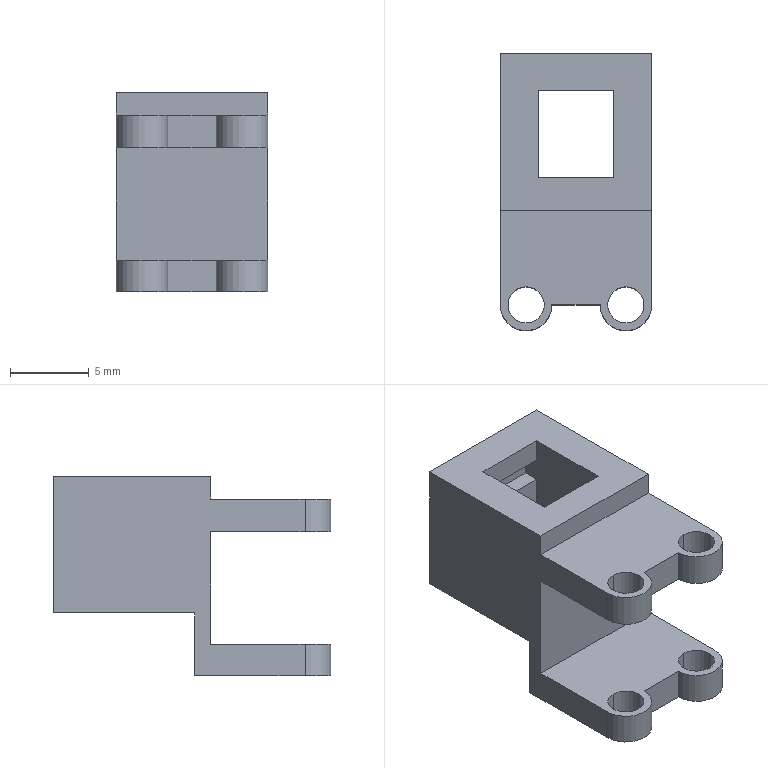Part | SolidWorks | features ICE 8, Extrusion 1 | 1 solid | 38 faces | box 9.63 x 17.64 x 12.7 mm | volume 865.254 mm3 | plane 26 | cylinder 12 | commonest cylinder face diameters 2.3 x8 3.28 x4
STEP:
#1=CARTESIAN_POINT('',(0.,1.15,7.242));
#2=VERTEX_POINT('',#1);
#3=CARTESIAN_POINT('',(0.,-1.15,7.242));
#4=VERTEX_POINT('',#3);
#5=CARTESIAN_POINT('',(0.,0.,7.242));
#6=DIRECTION('',(0.,0.,1.));
#7=DIRECTION('',(1.,0.,0.));
#8=AXIS2_PLACEMENT_3D('',#5,#6,#7);
#9=CIRCLE('',#8,1.15);
#10=EDGE_CURVE('',#2,#4,#9,.T.);
#11=ORIENTED_EDGE('',*,*,#10,.T.);
#12=CARTESIAN_POINT('',(0.,-1.15,5.171));
#13=VERTEX_POINT('',#12);
#14=CARTESIAN_POINT('',(0.,-1.15,8.7));
#15=DIRECTION('',(0.,0.,-1.));
#16=VECTOR('',#15,1000.);
#17=LINE('',#14,#16);
#18=EDGE_CURVE('',#4,#13,#17,.T.);
#19=ORIENTED_EDGE('',*,*,#18,.T.);
#20=CARTESIAN_POINT('',(0.,1.15,5.171));
#21=VERTEX_POINT('',#20);
#22=CARTESIAN_POINT('',(0.,0.,5.171));
#23=DIRECTION('',(0.,0.,-1.));
#24=DIRECTION('',(-1.,0.,0.));
#25=AXIS2_PLACEMENT_3D('',#22,#23,#24);
#26=CIRCLE('',#25,1.15);
#27=EDGE_CURVE('',#13,#21,#26,.T.);
#28=ORIENTED_EDGE('',*,*,#27,.T.);
#29=CARTESIAN_POINT('',(0.,1.15,8.7));
#30=DIRECTION('',(0.,0.,-1.));
#31=VECTOR('',#30,1000.);
#32=LINE('',#29,#31);
#33=EDGE_CURVE('',#2,#21,#32,.T.);
#34=ORIENTED_EDGE('',*,*,#33,.F.);
#35=EDGE_LOOP('',(#11,#19,#28,#34));
#36=FACE_OUTER_BOUND('',#35,.T.);
#37=CARTESIAN_POINT('',(0.,0.,8.7));
#38=DIRECTION('',(0.,0.,-1.));
#39=DIRECTION('',(0.,1.,0.));
#40=AXIS2_PLACEMENT_3D('',#37,#38,#39);
#41=CYLINDRICAL_SURFACE('',#40,1.15);
#42=ADVANCED_FACE('',(#36),#41,.F.);
#43=CARTESIAN_POINT('',(-6.35,1.15,7.242));
#44=VERTEX_POINT('',#43);
#45=CARTESIAN_POINT('',(-6.35,-1.15,7.242));
#46=VERTEX_POINT('',#45);
#47=CARTESIAN_POINT('',(-6.35,0.,7.242));
#48=DIRECTION('',(0.,0.,1.));
#49=DIRECTION('',(1.,0.,0.));
#50=AXIS2_PLACEMENT_3D('',#47,#48,#49);
#51=CIRCLE('',#50,1.15);
#52=EDGE_CURVE('',#44,#46,#51,.T.);
#53=ORIENTED_EDGE('',*,*,#52,.T.);
#54=CARTESIAN_POINT('',(-6.35,-1.15,5.171));
#55=VERTEX_POINT('',#54);
#56=CARTESIAN_POINT('',(-6.35,-1.15,8.7));
#57=DIRECTION('',(0.,0.,-1.));
#58=VECTOR('',#57,1000.);
#59=LINE('',#56,#58);
#60=EDGE_CURVE('',#46,#55,#59,.T.);
#61=ORIENTED_EDGE('',*,*,#60,.T.);
#62=CARTESIAN_POINT('',(-6.35,1.15,5.171));
#63=VERTEX_POINT('',#62);
#64=CARTESIAN_POINT('',(-6.35,0.,5.171));
#65=DIRECTION('',(0.,0.,-1.));
#66=DIRECTION('',(-1.,0.,0.));
#67=AXIS2_PLACEMENT_3D('',#64,#65,#66);
#68=CIRCLE('',#67,1.15);
#69=EDGE_CURVE('',#55,#63,#68,.T.);
#70=ORIENTED_EDGE('',*,*,#69,.T.);
#71=CARTESIAN_POINT('',(-6.35,1.15,8.7));
#72=DIRECTION('',(0.,0.,-1.));
#73=VECTOR('',#72,1000.);
#74=LINE('',#71,#73);
#75=EDGE_CURVE('',#44,#63,#74,.T.);
#76=ORIENTED_EDGE('',*,*,#75,.F.);
#77=EDGE_LOOP('',(#53,#61,#70,#76));
#78=FACE_OUTER_BOUND('',#77,.T.);
#79=CARTESIAN_POINT('',(-6.35,0.,8.7));
#80=DIRECTION('',(0.,0.,-1.));
#81=DIRECTION('',(0.,1.,0.));
#82=AXIS2_PLACEMENT_3D('',#79,#80,#81);
#83=CYLINDRICAL_SURFACE('',#82,1.15);
#84=ADVANCED_FACE('',(#78),#83,.F.);
#85=CARTESIAN_POINT('',(0.,1.15,-2.));
#86=VERTEX_POINT('',#85);
#87=CARTESIAN_POINT('',(0.,-1.15,-2.));
#88=VERTEX_POINT('',#87);
#89=CARTESIAN_POINT('',(0.,0.,-2.));
#90=DIRECTION('',(0.,0.,1.));
#91=DIRECTION('',(0.,-1.,0.));
#92=AXIS2_PLACEMENT_3D('',#89,#90,#91);
#93=CIRCLE('',#92,1.15);
#94=EDGE_CURVE('',#86,#88,#93,.T.);
#95=ORIENTED_EDGE('',*,*,#94,.T.);
#96=CARTESIAN_POINT('',(0.,-1.15,-4.));
#97=VERTEX_POINT('',#96);
#98=CARTESIAN_POINT('',(0.,-1.15,8.7));
#99=DIRECTION('',(0.,0.,-1.));
#100=VECTOR('',#99,1000.);
#101=LINE('',#98,#100);
#102=EDGE_CURVE('',#88,#97,#101,.T.);
#103=ORIENTED_EDGE('',*,*,#102,.T.);
#104=CARTESIAN_POINT('',(0.,1.15,-4.));
#105=VERTEX_POINT('',#104);
#106=CARTESIAN_POINT('',(0.,0.,-4.));
#107=DIRECTION('',(0.,0.,-1.));
#108=DIRECTION('',(0.,1.,0.));
#109=AXIS2_PLACEMENT_3D('',#106,#107,#108);
#110=CIRCLE('',#109,1.15);
#111=EDGE_CURVE('',#97,#105,#110,.T.);
#112=ORIENTED_EDGE('',*,*,#111,.T.);
#113=CARTESIAN_POINT('',(0.,1.15,8.7));
#114=DIRECTION('',(0.,0.,-1.));
#115=VECTOR('',#114,1000.);
#116=LINE('',#113,#115);
#117=EDGE_CURVE('',#86,#105,#116,.T.);
#118=ORIENTED_EDGE('',*,*,#117,.F.);
#119=EDGE_LOOP('',(#95,#103,#112,#118));
#120=FACE_OUTER_BOUND('',#119,.T.);
#121=CARTESIAN_POINT('',(0.,0.,8.7));
#122=DIRECTION('',(0.,0.,-1.));
#123=DIRECTION('',(0.,1.,0.));
#124=AXIS2_PLACEMENT_3D('',#121,#122,#123);
#125=CYLINDRICAL_SURFACE('',#124,1.15);
#126=ADVANCED_FACE('',(#120),#125,.F.);
#127=CARTESIAN_POINT('',(-6.35,1.15,-2.));
#128=VERTEX_POINT('',#127);
#129=CARTESIAN_POINT('',(-6.35,-1.15,-2.));
#130=VERTEX_POINT('',#129);
#131=CARTESIAN_POINT('',(-6.35,0.,-2.));
#132=DIRECTION('',(0.,0.,1.));
#133=DIRECTION('',(0.,-1.,0.));
#134=AXIS2_PLACEMENT_3D('',#131,#132,#133);
#135=CIRCLE('',#134,1.15);
#136=EDGE_CURVE('',#128,#130,#135,.T.);
#137=ORIENTED_EDGE('',*,*,#136,.T.);
#138=CARTESIAN_POINT('',(-6.35,-1.15,-4.));
#139=VERTEX_POINT('',#138);
#140=CARTESIAN_POINT('',(-6.35,-1.15,8.7));
#141=DIRECTION('',(0.,0.,-1.));
#142=VECTOR('',#141,1000.);
#143=LINE('',#140,#142);
#144=EDGE_CURVE('',#130,#139,#143,.T.);
#145=ORIENTED_EDGE('',*,*,#144,.T.);
#146=CARTESIAN_POINT('',(-6.35,1.15,-4.));
#147=VERTEX_POINT('',#146);
#148=CARTESIAN_POINT('',(-6.35,0.,-4.));
#149=DIRECTION('',(0.,0.,-1.));
#150=DIRECTION('',(0.,1.,0.));
#151=AXIS2_PLACEMENT_3D('',#148,#149,#150);
#152=CIRCLE('',#151,1.15);
#153=EDGE_CURVE('',#139,#147,#152,.T.);
#154=ORIENTED_EDGE('',*,*,#153,.T.);
#155=CARTESIAN_POINT('',(-6.35,1.15,8.7));
#156=DIRECTION('',(0.,0.,-1.));
#157=VECTOR('',#156,1000.);
#158=LINE('',#155,#157);
#159=EDGE_CURVE('',#128,#147,#158,.T.);
#160=ORIENTED_EDGE('',*,*,#159,.F.);
#161=EDGE_LOOP('',(#137,#145,#154,#160));
#162=FACE_OUTER_BOUND('',#161,.T.);
#163=CARTESIAN_POINT('',(-6.35,0.,8.7));
#164=DIRECTION('',(0.,0.,-1.));
#165=DIRECTION('',(0.,1.,0.));
#166=AXIS2_PLACEMENT_3D('',#163,#164,#165);
#167=CYLINDRICAL_SURFACE('',#166,1.15);
#168=ADVANCED_FACE('',(#162),#167,.F.);
#169=CARTESIAN_POINT('',(0.,0.,5.171));
#170=DIRECTION('',(0.,0.,-1.));
#171=DIRECTION('',(-1.,0.,0.));
#172=AXIS2_PLACEMENT_3D('',#169,#170,#171);
#173=CIRCLE('',#172,1.15);
#174=EDGE_CURVE('',#21,#13,#173,.T.);
#175=ORIENTED_EDGE('',*,*,#174,.F.);
#176=ORIENTED_EDGE('',*,*,#27,.F.);
#177=EDGE_LOOP('',(#175,#176));
#178=FACE_BOUND('',#177,.T.);
#179=CARTESIAN_POINT('',(-6.35,0.,5.171));
#180=DIRECTION('',(0.,0.,-1.));
#181=DIRECTION('',(-1.,0.,0.));
#182=AXIS2_PLACEMENT_3D('',#179,#180,#181);
#183=CIRCLE('',#182,1.15);
#184=EDGE_CURVE('',#63,#55,#183,.T.);
#185=ORIENTED_EDGE('',*,*,#184,.F.);
#186=ORIENTED_EDGE('',*,*,#69,.F.);
#187=EDGE_LOOP('',(#185,#186));
#188=FACE_BOUND('',#187,.T.);
#189=CARTESIAN_POINT('',(1.64,6.,5.171));
#190=VERTEX_POINT('',#189);
#191=CARTESIAN_POINT('',(1.64,0.,5.171));
#192=VERTEX_POINT('',#191);
#193=CARTESIAN_POINT('',(1.64,-1.64,5.171));
#194=DIRECTION('',(0.,-1.,0.));
#195=VECTOR('',#194,1000.);
#196=LINE('',#193,#195);
#197=EDGE_CURVE('',#190,#192,#196,.T.);
#198=ORIENTED_EDGE('',*,*,#197,.T.);
#199=CARTESIAN_POINT('',(-1.64,0.,5.171));
#200=VERTEX_POINT('',#199);
#201=CARTESIAN_POINT('',(0.,0.,5.171));
#202=DIRECTION('',(0.,0.,-1.));
#203=DIRECTION('',(-1.,0.,0.));
#204=AXIS2_PLACEMENT_3D('',#201,#202,#203);
#205=CIRCLE('',#204,1.64);
#206=EDGE_CURVE('',#192,#200,#205,.T.);
#207=ORIENTED_EDGE('',*,*,#206,.T.);
#208=CARTESIAN_POINT('',(-4.71,0.,5.171));
#209=VERTEX_POINT('',#208);
#210=CARTESIAN_POINT('',(11.161,0.,5.171));
#211=DIRECTION('',(-1.,0.,0.));
#212=VECTOR('',#211,1000.);
#213=LINE('',#210,#212);
#214=EDGE_CURVE('',#200,#209,#213,.T.);
#215=ORIENTED_EDGE('',*,*,#214,.T.);
#216=CARTESIAN_POINT('',(-7.99,0.,5.171));
#217=VERTEX_POINT('',#216);
#218=CARTESIAN_POINT('',(-6.35,0.,5.171));
#219=DIRECTION('',(0.,0.,-1.));
#220=DIRECTION('',(-1.,0.,0.));
#221=AXIS2_PLACEMENT_3D('',#218,#219,#220);
#222=CIRCLE('',#221,1.64);
#223=EDGE_CURVE('',#209,#217,#222,.T.);
#224=ORIENTED_EDGE('',*,*,#223,.T.);
#225=CARTESIAN_POINT('',(-7.99,6.,5.171));
#226=VERTEX_POINT('',#225);
#227=CARTESIAN_POINT('',(-7.99,-1.64,5.171));
#228=DIRECTION('',(0.,-1.,0.));
#229=VECTOR('',#228,1000.);
#230=LINE('',#227,#229);
#231=EDGE_CURVE('',#226,#217,#230,.T.);
#232=ORIENTED_EDGE('',*,*,#231,.F.);
#233=CARTESIAN_POINT('',(11.161,6.,5.171));
#234=DIRECTION('',(-1.,0.,0.));
#235=VECTOR('',#234,1000.);
#236=LINE('',#233,#235);
#237=EDGE_CURVE('',#190,#226,#236,.T.);
#238=ORIENTED_EDGE('',*,*,#237,.F.);
#239=EDGE_LOOP('',(#198,#207,#215,#224,#232,#238));
#240=FACE_OUTER_BOUND('',#239,.T.);
#241=CARTESIAN_POINT('',(11.161,-1.64,5.171));
#242=DIRECTION('',(0.,0.,-1.));
#243=DIRECTION('',(-1.,0.,0.));
#244=AXIS2_PLACEMENT_3D('',#241,#242,#243);
#245=PLANE('',#244);
#246=ADVANCED_FACE('',(#178,#188,#240),#245,.T.);
#247=ORIENTED_EDGE('',*,*,#10,.F.);
#248=CARTESIAN_POINT('',(0.,0.,7.242));
#249=DIRECTION('',(0.,0.,1.));
#250=DIRECTION('',(1.,0.,0.));
#251=AXIS2_PLACEMENT_3D('',#248,#249,#250);
#252=CIRCLE('',#251,1.15);
#253=EDGE_CURVE('',#4,#2,#252,.T.);
#254=ORIENTED_EDGE('',*,*,#253,.F.);
#255=EDGE_LOOP('',(#247,#254));
#256=FACE_BOUND('',#255,.T.);
#257=ORIENTED_EDGE('',*,*,#52,.F.);
#258=CARTESIAN_POINT('',(-6.35,0.,7.242));
#259=DIRECTION('',(0.,0.,1.));
#260=DIRECTION('',(1.,0.,0.));
#261=AXIS2_PLACEMENT_3D('',#258,#259,#260);
#262=CIRCLE('',#261,1.15);
#263=EDGE_CURVE('',#46,#44,#262,.T.);
#264=ORIENTED_EDGE('',*,*,#263,.F.);
#265=EDGE_LOOP('',(#257,#264));
#266=FACE_BOUND('',#265,.T.);
#267=CARTESIAN_POINT('',(-1.64,0.,7.242));
#268=VERTEX_POINT('',#267);
#269=CARTESIAN_POINT('',(1.64,0.,7.242));
#270=VERTEX_POINT('',#269);
#271=CARTESIAN_POINT('',(0.,0.,7.242));
#272=DIRECTION('',(0.,0.,1.));
#273=DIRECTION('',(1.,0.,0.));
#274=AXIS2_PLACEMENT_3D('',#271,#272,#273);
#275=CIRCLE('',#274,1.64);
#276=EDGE_CURVE('',#268,#270,#275,.T.);
#277=ORIENTED_EDGE('',*,*,#276,.T.);
#278=CARTESIAN_POINT('',(1.64,6.,7.242));
#279=VERTEX_POINT('',#278);
#280=CARTESIAN_POINT('',(1.64,6.,7.242));
#281=DIRECTION('',(0.,1.,0.));
#282=VECTOR('',#281,1000.);
#283=LINE('',#280,#282);
#284=EDGE_CURVE('',#270,#279,#283,.T.);
#285=ORIENTED_EDGE('',*,*,#284,.T.);
#286=CARTESIAN_POINT('',(-7.99,6.,7.242));
#287=VERTEX_POINT('',#286);
#288=CARTESIAN_POINT('',(11.161,6.,7.242));
#289=DIRECTION('',(-1.,0.,0.));
#290=VECTOR('',#289,1000.);
#291=LINE('',#288,#290);
#292=EDGE_CURVE('',#279,#287,#291,.T.);
#293=ORIENTED_EDGE('',*,*,#292,.T.);
#294=CARTESIAN_POINT('',(-7.99,0.,7.242));
#295=VERTEX_POINT('',#294);
#296=CARTESIAN_POINT('',(-7.99,6.,7.242));
#297=DIRECTION('',(0.,1.,0.));
#298=VECTOR('',#297,1000.);
#299=LINE('',#296,#298);
#300=EDGE_CURVE('',#295,#287,#299,.T.);
#301=ORIENTED_EDGE('',*,*,#300,.F.);
#302=CARTESIAN_POINT('',(-4.71,0.,7.242));
#303=VERTEX_POINT('',#302);
#304=CARTESIAN_POINT('',(-6.35,0.,7.242));
#305=DIRECTION('',(0.,0.,1.));
#306=DIRECTION('',(1.,0.,0.));
#307=AXIS2_PLACEMENT_3D('',#304,#305,#306);
#308=CIRCLE('',#307,1.64);
#309=EDGE_CURVE('',#295,#303,#308,.T.);
#310=ORIENTED_EDGE('',*,*,#309,.T.);
#311=CARTESIAN_POINT('',(11.161,0.,7.242));
#312=DIRECTION('',(1.,0.,0.));
#313=VECTOR('',#312,1000.);
#314=LINE('',#311,#313);
#315=EDGE_CURVE('',#303,#268,#314,.T.);
#316=ORIENTED_EDGE('',*,*,#315,.T.);
#317=EDGE_LOOP('',(#277,#285,#293,#301,#310,#316));
#318=FACE_OUTER_BOUND('',#317,.T.);
#319=CARTESIAN_POINT('',(11.161,6.,7.242));
#320=DIRECTION('',(0.,0.,1.));
#321=DIRECTION('',(1.,0.,0.));
#322=AXIS2_PLACEMENT_3D('',#319,#320,#321);
#323=PLANE('',#322);
#324=ADVANCED_FACE('',(#256,#266,#318),#323,.T.);
#325=CARTESIAN_POINT('',(0.,0.,-4.));
#326=DIRECTION('',(0.,0.,-1.));
#327=DIRECTION('',(0.,1.,0.));
#328=AXIS2_PLACEMENT_3D('',#325,#326,#327);
#329=CIRCLE('',#328,1.15);
#330=EDGE_CURVE('',#105,#97,#329,.T.);
#331=ORIENTED_EDGE('',*,*,#330,.F.);
#332=ORIENTED_EDGE('',*,*,#111,.F.);
#333=EDGE_LOOP('',(#331,#332));
#334=FACE_BOUND('',#333,.T.);
#335=CARTESIAN_POINT('',(-6.35,0.,-4.));
#336=DIRECTION('',(0.,0.,-1.));
#337=DIRECTION('',(0.,1.,0.));
#338=AXIS2_PLACEMENT_3D('',#335,#336,#337);
#339=CIRCLE('',#338,1.15);
#340=EDGE_CURVE('',#147,#139,#339,.T.);
#341=ORIENTED_EDGE('',*,*,#340,.F.);
#342=ORIENTED_EDGE('',*,*,#153,.F.);
#343=EDGE_LOOP('',(#341,#342));
#344=FACE_BOUND('',#343,.T.);
#345=CARTESIAN_POINT('',(1.64,7.,-4.));
#346=VERTEX_POINT('',#345);
#347=CARTESIAN_POINT('',(1.64,0.,-4.));
#348=VERTEX_POINT('',#347);
#349=CARTESIAN_POINT('',(1.64,6.,-4.));
#350=DIRECTION('',(0.,-1.,0.));
#351=VECTOR('',#350,1000.);
#352=LINE('',#349,#351);
#353=EDGE_CURVE('',#346,#348,#352,.T.);
#354=ORIENTED_EDGE('',*,*,#353,.T.);
#355=CARTESIAN_POINT('',(-1.64,0.,-4.));
#356=VERTEX_POINT('',#355);
#357=CARTESIAN_POINT('',(0.,0.,-4.));
#358=DIRECTION('',(0.,0.,-1.));
#359=DIRECTION('',(0.,1.,0.));
#360=AXIS2_PLACEMENT_3D('',#357,#358,#359);
#361=CIRCLE('',#360,1.64);
#362=EDGE_CURVE('',#348,#356,#361,.T.);
#363=ORIENTED_EDGE('',*,*,#362,.T.);
#364=CARTESIAN_POINT('',(-4.71,0.,-4.));
#365=VERTEX_POINT('',#364);
#366=CARTESIAN_POINT('',(0.,0.,-4.));
#367=DIRECTION('',(-1.,0.,0.));
#368=VECTOR('',#367,1000.);
#369=LINE('',#366,#368);
#370=EDGE_CURVE('',#356,#365,#369,.T.);
#371=ORIENTED_EDGE('',*,*,#370,.T.);
#372=CARTESIAN_POINT('',(-7.99,0.,-4.));
#373=VERTEX_POINT('',#372);
#374=CARTESIAN_POINT('',(-6.35,0.,-4.));
#375=DIRECTION('',(0.,0.,-1.));
#376=DIRECTION('',(0.,1.,0.));
#377=AXIS2_PLACEMENT_3D('',#374,#375,#376);
#378=CIRCLE('',#377,1.64);
#379=EDGE_CURVE('',#365,#373,#378,.T.);
#380=ORIENTED_EDGE('',*,*,#379,.T.);
#381=CARTESIAN_POINT('',(-7.99,7.,-4.));
#382=VERTEX_POINT('',#381);
#383=CARTESIAN_POINT('',(-7.99,6.,-4.));
#384=DIRECTION('',(0.,-1.,0.));
#385=VECTOR('',#384,1000.);
#386=LINE('',#383,#385);
#387=EDGE_CURVE('',#382,#373,#386,.T.);
#388=ORIENTED_EDGE('',*,*,#387,.F.);
#389=CARTESIAN_POINT('',(11.161,7.,-4.));
#390=DIRECTION('',(-1.,0.,0.));
#391=VECTOR('',#390,1000.);
#392=LINE('',#389,#391);
#393=EDGE_CURVE('',#346,#382,#392,.T.);
#394=ORIENTED_EDGE('',*,*,#393,.F.);
#395=EDGE_LOOP('',(#354,#363,#371,#380,#388,#394));
#396=FACE_OUTER_BOUND('',#395,.T.);
#397=CARTESIAN_POINT('',(11.161,6.,-4.));
#398=DIRECTION('',(0.,0.,-1.));
#399=DIRECTION('',(0.,1.,0.));
#400=AXIS2_PLACEMENT_3D('',#397,#398,#399);
#401=PLANE('',#400);
#402=ADVANCED_FACE('',(#334,#344,#396),#401,.T.);
#403=ORIENTED_EDGE('',*,*,#94,.F.);
#404=CARTESIAN_POINT('',(0.,0.,-2.));
#405=DIRECTION('',(0.,0.,1.));
#406=DIRECTION('',(0.,-1.,0.));
#407=AXIS2_PLACEMENT_3D('',#404,#405,#406);
#408=CIRCLE('',#407,1.15);
#409=EDGE_CURVE('',#88,#86,#408,.T.);
#410=ORIENTED_EDGE('',*,*,#409,.F.);
#411=EDGE_LOOP('',(#403,#410));
#412=FACE_BOUND('',#411,.T.);
#413=ORIENTED_EDGE('',*,*,#136,.F.);
#414=CARTESIAN_POINT('',(-6.35,0.,-2.));
#415=DIRECTION('',(0.,0.,1.));
#416=DIRECTION('',(0.,-1.,0.));
#417=AXIS2_PLACEMENT_3D('',#414,#415,#416);
#418=CIRCLE('',#417,1.15);
#419=EDGE_CURVE('',#130,#128,#418,.T.);
#420=ORIENTED_EDGE('',*,*,#419,.F.);
#421=EDGE_LOOP('',(#413,#420));
#422=FACE_BOUND('',#421,.T.);
#423=CARTESIAN_POINT('',(-1.64,0.,-2.));
#424=VERTEX_POINT('',#423);
#425=CARTESIAN_POINT('',(1.64,0.,-2.));
#426=VERTEX_POINT('',#425);
#427=CARTESIAN_POINT('',(0.,0.,-2.));
#428=DIRECTION('',(0.,0.,1.));
#429=DIRECTION('',(0.,-1.,0.));
#430=AXIS2_PLACEMENT_3D('',#427,#428,#429);
#431=CIRCLE('',#430,1.64);
#432=EDGE_CURVE('',#424,#426,#431,.T.);
#433=ORIENTED_EDGE('',*,*,#432,.T.);
#434=CARTESIAN_POINT('',(1.64,6.,-2.));
#435=VERTEX_POINT('',#434);
#436=CARTESIAN_POINT('',(1.64,6.,-2.));
#437=DIRECTION('',(0.,1.,0.));
#438=VECTOR('',#437,1000.);
#439=LINE('',#436,#438);
#440=EDGE_CURVE('',#426,#435,#439,.T.);
#441=ORIENTED_EDGE('',*,*,#440,.T.);
#442=CARTESIAN_POINT('',(-7.99,6.,-2.));
#443=VERTEX_POINT('',#442);
#444=CARTESIAN_POINT('',(11.161,6.,-2.));
#445=DIRECTION('',(-1.,0.,0.));
#446=VECTOR('',#445,1000.);
#447=LINE('',#444,#446);
#448=EDGE_CURVE('',#435,#443,#447,.T.);
#449=ORIENTED_EDGE('',*,*,#448,.T.);
#450=CARTESIAN_POINT('',(-7.99,0.,-2.));
#451=VERTEX_POINT('',#450);
#452=CARTESIAN_POINT('',(-7.99,6.,-2.));
#453=DIRECTION('',(0.,1.,0.));
#454=VECTOR('',#453,1000.);
#455=LINE('',#452,#454);
#456=EDGE_CURVE('',#451,#443,#455,.T.);
#457=ORIENTED_EDGE('',*,*,#456,.F.);
#458=CARTESIAN_POINT('',(-4.71,0.,-2.));
#459=VERTEX_POINT('',#458);
#460=CARTESIAN_POINT('',(-6.35,0.,-2.));
#461=DIRECTION('',(0.,0.,1.));
#462=DIRECTION('',(0.,-1.,0.));
#463=AXIS2_PLACEMENT_3D('',#460,#461,#462);
#464=CIRCLE('',#463,1.64);
#465=EDGE_CURVE('',#451,#459,#464,.T.);
#466=ORIENTED_EDGE('',*,*,#465,.T.);
#467=CARTESIAN_POINT('',(11.161,0.,-2.));
#468=DIRECTION('',(1.,0.,0.));
#469=VECTOR('',#468,1000.);
#470=LINE('',#467,#469);
#471=EDGE_CURVE('',#459,#424,#470,.T.);
#472=ORIENTED_EDGE('',*,*,#471,.T.);
#473=EDGE_LOOP('',(#433,#441,#449,#457,#466,#472));
#474=FACE_OUTER_BOUND('',#473,.T.);
#475=CARTESIAN_POINT('',(11.161,6.,-2.));
#476=DIRECTION('',(0.,0.,1.));
#477=DIRECTION('',(0.,-1.,0.));
#478=AXIS2_PLACEMENT_3D('',#475,#476,#477);
#479=PLANE('',#478);
#480=ADVANCED_FACE('',(#412,#422,#474),#479,.T.);
#481=ORIENTED_EDGE('',*,*,#284,.F.);
#482=CARTESIAN_POINT('',(1.64,0.,8.7));
#483=DIRECTION('',(0.,0.,-1.));
#484=VECTOR('',#483,1000.);
#485=LINE('',#482,#484);
#486=EDGE_CURVE('',#270,#192,#485,.T.);
#487=ORIENTED_EDGE('',*,*,#486,.T.);
#488=ORIENTED_EDGE('',*,*,#197,.F.);
#489=CARTESIAN_POINT('',(1.64,6.,8.7));
#490=DIRECTION('',(0.,0.,-1.));
#491=VECTOR('',#490,1000.);
#492=LINE('',#489,#491);
#493=EDGE_CURVE('',#190,#435,#492,.T.);
#494=ORIENTED_EDGE('',*,*,#493,.T.);
#495=ORIENTED_EDGE('',*,*,#440,.F.);
#496=CARTESIAN_POINT('',(1.64,0.,8.7));
#497=DIRECTION('',(0.,0.,-1.));
#498=VECTOR('',#497,1000.);
#499=LINE('',#496,#498);
#500=EDGE_CURVE('',#426,#348,#499,.T.);
#501=ORIENTED_EDGE('',*,*,#500,.T.);
#502=ORIENTED_EDGE('',*,*,#353,.F.);
#503=CARTESIAN_POINT('',(1.64,7.,0.));
#504=VERTEX_POINT('',#503);
#505=CARTESIAN_POINT('',(1.64,7.,-4.));
#506=DIRECTION('',(0.,0.,-1.));
#507=VECTOR('',#506,1000.);
#508=LINE('',#505,#507);
#509=EDGE_CURVE('',#504,#346,#508,.T.);
#510=ORIENTED_EDGE('',*,*,#509,.F.);
#511=CARTESIAN_POINT('',(1.64,16.,0.));
#512=VERTEX_POINT('',#511);
#513=CARTESIAN_POINT('',(1.64,0.,0.));
#514=DIRECTION('',(0.,1.,0.));
#515=VECTOR('',#514,1000.);
#516=LINE('',#513,#515);
#517=EDGE_CURVE('',#504,#512,#516,.T.);
#518=ORIENTED_EDGE('',*,*,#517,.T.);
#519=CARTESIAN_POINT('',(1.64,16.,8.7));
#520=VERTEX_POINT('',#519);
#521=CARTESIAN_POINT('',(1.64,16.,-18.674));
#522=DIRECTION('',(0.,0.,1.));
#523=VECTOR('',#522,1000.);
#524=LINE('',#521,#523);
#525=EDGE_CURVE('',#512,#520,#524,.T.);
#526=ORIENTED_EDGE('',*,*,#525,.T.);
#527=CARTESIAN_POINT('',(1.64,6.,8.7));
#528=VERTEX_POINT('',#527);
#529=CARTESIAN_POINT('',(1.64,16.,8.7));
#530=DIRECTION('',(0.,1.,0.));
#531=VECTOR('',#530,1000.);
#532=LINE('',#529,#531);
#533=EDGE_CURVE('',#528,#520,#532,.T.);
#534=ORIENTED_EDGE('',*,*,#533,.F.);
#535=CARTESIAN_POINT('',(1.64,6.,8.7));
#536=DIRECTION('',(0.,0.,-1.));
#537=VECTOR('',#536,1000.);
#538=LINE('',#535,#537);
#539=EDGE_CURVE('',#528,#279,#538,.T.);
#540=ORIENTED_EDGE('',*,*,#539,.T.);
#541=EDGE_LOOP('',(#481,#487,#488,#494,#495,#501,#502,#510,#518,#526,#534,#540));
#542=FACE_OUTER_BOUND('',#541,.T.);
#543=CARTESIAN_POINT('',(1.64,0.,-18.674));
#544=DIRECTION('',(1.,0.,0.));
#545=DIRECTION('',(0.,0.,-1.));
#546=AXIS2_PLACEMENT_3D('',#543,#544,#545);
#547=PLANE('',#546);
#548=ADVANCED_FACE('',(#542),#547,.T.);
#549=ORIENTED_EDGE('',*,*,#493,.F.);
#550=ORIENTED_EDGE('',*,*,#237,.T.);
#551=CARTESIAN_POINT('',(-7.99,6.,8.7));
#552=DIRECTION('',(0.,0.,-1.));
#553=VECTOR('',#552,1000.);
#554=LINE('',#551,#553);
#555=EDGE_CURVE('',#226,#443,#554,.T.);
#556=ORIENTED_EDGE('',*,*,#555,.T.);
#557=ORIENTED_EDGE('',*,*,#448,.F.);
#558=EDGE_LOOP('',(#549,#550,#556,#557));
#559=FACE_OUTER_BOUND('',#558,.T.);
#560=CARTESIAN_POINT('',(-7.99,6.,8.7));
#561=DIRECTION('',(0.,1.,0.));
#562=DIRECTION('',(0.,0.,1.));
#563=AXIS2_PLACEMENT_3D('',#560,#561,#562);
#564=PLANE('',#563);
#565=ADVANCED_FACE('',(#559),#564,.F.);
#566=CARTESIAN_POINT('',(-0.76,13.615,7.2));
#567=VERTEX_POINT('',#566);
#568=CARTESIAN_POINT('',(-5.59,13.615,7.2));
#569=VERTEX_POINT('',#568);
#570=CARTESIAN_POINT('',(-5.59,13.615,7.2));
#571=DIRECTION('',(-1.,0.,0.));
#572=VECTOR('',#571,1000.);
#573=LINE('',#570,#572);
#574=EDGE_CURVE('',#567,#569,#573,.T.);
#575=ORIENTED_EDGE('',*,*,#574,.F.);
#576=CARTESIAN_POINT('',(-0.76,13.615,8.7));
#577=VERTEX_POINT('',#576);
#578=CARTESIAN_POINT('',(-0.76,13.615,-1.3));
#579=DIRECTION('',(0.,0.,1.));
#580=VECTOR('',#579,1000.);
#581=LINE('',#578,#580);
#582=EDGE_CURVE('',#567,#577,#581,.T.);
#583=ORIENTED_EDGE('',*,*,#582,.T.);
#584=CARTESIAN_POINT('',(-5.59,13.615,8.7));
#585=VERTEX_POINT('',#584);
#586=CARTESIAN_POINT('',(-5.59,13.615,8.7));
#587=DIRECTION('',(-1.,0.,0.));
#588=VECTOR('',#587,1000.);
#589=LINE('',#586,#588);
#590=EDGE_CURVE('',#577,#585,#589,.T.);
#591=ORIENTED_EDGE('',*,*,#590,.T.);
#592=CARTESIAN_POINT('',(-5.59,13.615,-1.3));
#593=DIRECTION('',(0.,0.,1.));
#594=VECTOR('',#593,1000.);
#595=LINE('',#592,#594);
#596=EDGE_CURVE('',#569,#585,#595,.T.);
#597=ORIENTED_EDGE('',*,*,#596,.F.);
#598=EDGE_LOOP('',(#575,#583,#591,#597));
#599=FACE_OUTER_BOUND('',#598,.T.);
#600=CARTESIAN_POINT('',(-5.59,13.615,-1.3));
#601=DIRECTION('',(0.,1.,0.));
#602=DIRECTION('',(-1.,0.,0.));
#603=AXIS2_PLACEMENT_3D('',#600,#601,#602);
#604=PLANE('',#603);
#605=ADVANCED_FACE('',(#599),#604,.F.);
#606=CARTESIAN_POINT('',(-5.59,8.085,7.2));
#607=VERTEX_POINT('',#606);
#608=CARTESIAN_POINT('',(-0.76,8.085,7.2));
#609=VERTEX_POINT('',#608);
#610=CARTESIAN_POINT('',(-5.59,8.085,7.2));
#611=DIRECTION('',(1.,0.,0.));
#612=VECTOR('',#611,1000.);
#613=LINE('',#610,#612);
#614=EDGE_CURVE('',#607,#609,#613,.T.);
#615=ORIENTED_EDGE('',*,*,#614,.F.);
#616=CARTESIAN_POINT('',(-5.59,8.085,8.7));
#617=VERTEX_POINT('',#616);
#618=CARTESIAN_POINT('',(-5.59,8.085,-1.3));
#619=DIRECTION('',(0.,0.,1.));
#620=VECTOR('',#619,1000.);
#621=LINE('',#618,#620);
#622=EDGE_CURVE('',#607,#617,#621,.T.);
#623=ORIENTED_EDGE('',*,*,#622,.T.);
#624=CARTESIAN_POINT('',(-0.76,8.085,8.7));
#625=VERTEX_POINT('',#624);
#626=CARTESIAN_POINT('',(-5.59,8.085,8.7));
#627=DIRECTION('',(1.,0.,0.));
#628=VECTOR('',#627,1000.);
#629=LINE('',#626,#628);
#630=EDGE_CURVE('',#617,#625,#629,.T.);
#631=ORIENTED_EDGE('',*,*,#630,.T.);
#632=CARTESIAN_POINT('',(-0.76,8.085,-1.3));
#633=DIRECTION('',(0.,0.,1.));
#634=VECTOR('',#633,1000.);
#635=LINE('',#632,#634);
#636=EDGE_CURVE('',#609,#625,#635,.T.);
#637=ORIENTED_EDGE('',*,*,#636,.F.);
#638=EDGE_LOOP('',(#615,#623,#631,#637));
#639=FACE_OUTER_BOUND('',#638,.T.);
#640=CARTESIAN_POINT('',(-5.59,8.085,-1.3));
#641=DIRECTION('',(0.,-1.,0.));
#642=DIRECTION('',(0.,0.,-1.));
#643=AXIS2_PLACEMENT_3D('',#640,#641,#642);
#644=PLANE('',#643);
#645=ADVANCED_FACE('',(#639),#644,.F.);
#646=CARTESIAN_POINT('',(-0.76,13.615,0.));
#647=VERTEX_POINT('',#646);
#648=CARTESIAN_POINT('',(-5.59,13.615,0.));
#649=VERTEX_POINT('',#648);
#650=CARTESIAN_POINT('',(0.,13.615,0.));
#651=DIRECTION('',(-1.,0.,0.));
#652=VECTOR('',#651,1000.);
#653=LINE('',#650,#652);
#654=EDGE_CURVE('',#647,#649,#653,.T.);
#655=ORIENTED_EDGE('',*,*,#654,.T.);
#656=CARTESIAN_POINT('',(-5.59,8.085,0.));
#657=VERTEX_POINT('',#656);
#658=CARTESIAN_POINT('',(-5.59,0.,0.));
#659=DIRECTION('',(0.,-1.,0.));
#660=VECTOR('',#659,1000.);
#661=LINE('',#658,#660);
#662=EDGE_CURVE('',#649,#657,#661,.T.);
#663=ORIENTED_EDGE('',*,*,#662,.T.);
#664=CARTESIAN_POINT('',(-0.76,8.085,0.));
#665=VERTEX_POINT('',#664);
#666=CARTESIAN_POINT('',(0.,8.085,0.));
#667=DIRECTION('',(1.,0.,0.));
#668=VECTOR('',#667,1000.);
#669=LINE('',#666,#668);
#670=EDGE_CURVE('',#657,#665,#669,.T.);
#671=ORIENTED_EDGE('',*,*,#670,.T.);
#672=CARTESIAN_POINT('',(-0.76,0.,0.));
#673=DIRECTION('',(0.,1.,0.));
#674=VECTOR('',#673,1000.);
#675=LINE('',#672,#674);
#676=EDGE_CURVE('',#665,#647,#675,.T.);
#677=ORIENTED_EDGE('',*,*,#676,.T.);
#678=EDGE_LOOP('',(#655,#663,#671,#677));
#679=FACE_BOUND('',#678,.T.);
#680=ORIENTED_EDGE('',*,*,#517,.F.);
#681=CARTESIAN_POINT('',(-7.99,7.,0.));
#682=VERTEX_POINT('',#681);
#683=CARTESIAN_POINT('',(11.161,7.,0.));
#684=DIRECTION('',(-1.,0.,0.));
#685=VECTOR('',#684,1000.);
#686=LINE('',#683,#685);
#687=EDGE_CURVE('',#504,#682,#686,.T.);
#688=ORIENTED_EDGE('',*,*,#687,.T.);
#689=CARTESIAN_POINT('',(-7.99,16.,0.));
#690=VERTEX_POINT('',#689);
#691=CARTESIAN_POINT('',(-7.99,0.,0.));
#692=DIRECTION('',(0.,-1.,0.));
#693=VECTOR('',#692,1000.);
#694=LINE('',#691,#693);
#695=EDGE_CURVE('',#690,#682,#694,.T.);
#696=ORIENTED_EDGE('',*,*,#695,.F.);
#697=CARTESIAN_POINT('',(1.64,16.,0.));
#698=DIRECTION('',(-1.,0.,0.));
#699=VECTOR('',#698,1000.);
#700=LINE('',#697,#699);
#701=EDGE_CURVE('',#512,#690,#700,.T.);
#702=ORIENTED_EDGE('',*,*,#701,.F.);
#703=EDGE_LOOP('',(#680,#688,#696,#702));
#704=FACE_OUTER_BOUND('',#703,.T.);
#705=CARTESIAN_POINT('',(0.,0.,0.));
#706=DIRECTION('',(0.,0.,1.));
#707=DIRECTION('',(1.,0.,0.));
#708=AXIS2_PLACEMENT_3D('',#705,#706,#707);
#709=PLANE('',#708);
#710=ADVANCED_FACE('',(#679,#704),#709,.F.);
#711=ORIENTED_EDGE('',*,*,#525,.F.);
#712=ORIENTED_EDGE('',*,*,#701,.T.);
#713=CARTESIAN_POINT('',(-7.99,16.,8.7));
#714=VERTEX_POINT('',#713);
#715=CARTESIAN_POINT('',(-7.99,16.,-18.674));
#716=DIRECTION('',(0.,0.,1.));
#717=VECTOR('',#716,1000.);
#718=LINE('',#715,#717);
#719=EDGE_CURVE('',#690,#714,#718,.T.);
#720=ORIENTED_EDGE('',*,*,#719,.T.);
#721=CARTESIAN_POINT('',(-7.99,16.,8.7));
#722=DIRECTION('',(-1.,0.,0.));
#723=VECTOR('',#722,1000.);
#724=LINE('',#721,#723);
#725=EDGE_CURVE('',#520,#714,#724,.T.);
#726=ORIENTED_EDGE('',*,*,#725,.F.);
#727=EDGE_LOOP('',(#711,#712,#720,#726));
#728=FACE_OUTER_BOUND('',#727,.T.);
#729=CARTESIAN_POINT('',(1.64,16.,-18.674));
#730=DIRECTION('',(0.,1.,0.));
#731=DIRECTION('',(0.,0.,1.));
#732=AXIS2_PLACEMENT_3D('',#729,#730,#731);
#733=PLANE('',#732);
#734=ADVANCED_FACE('',(#728),#733,.T.);
#735=CARTESIAN_POINT('',(-7.99,0.,8.7));
#736=DIRECTION('',(0.,0.,-1.));
#737=VECTOR('',#736,1000.);
#738=LINE('',#735,#737);
#739=EDGE_CURVE('',#295,#217,#738,.T.);
#740=ORIENTED_EDGE('',*,*,#739,.F.);
#741=ORIENTED_EDGE('',*,*,#300,.T.);
#742=CARTESIAN_POINT('',(-7.99,6.,8.7));
#743=VERTEX_POINT('',#742);
#744=CARTESIAN_POINT('',(-7.99,6.,8.7));
#745=DIRECTION('',(0.,0.,-1.));
#746=VECTOR('',#745,1000.);
#747=LINE('',#744,#746);
#748=EDGE_CURVE('',#743,#287,#747,.T.);
#749=ORIENTED_EDGE('',*,*,#748,.F.);
#750=CARTESIAN_POINT('',(-7.99,16.,8.7));
#751=DIRECTION('',(0.,-1.,0.));
#752=VECTOR('',#751,1000.);
#753=LINE('',#750,#752);
#754=EDGE_CURVE('',#714,#743,#753,.T.);
#755=ORIENTED_EDGE('',*,*,#754,.F.);
#756=ORIENTED_EDGE('',*,*,#719,.F.);
#757=ORIENTED_EDGE('',*,*,#695,.T.);
#758=CARTESIAN_POINT('',(-7.99,7.,-4.));
#759=DIRECTION('',(0.,0.,-1.));
#760=VECTOR('',#759,1000.);
#761=LINE('',#758,#760);
#762=EDGE_CURVE('',#682,#382,#761,.T.);
#763=ORIENTED_EDGE('',*,*,#762,.T.);
#764=ORIENTED_EDGE('',*,*,#387,.T.);
#765=CARTESIAN_POINT('',(-7.99,0.,8.7));
#766=DIRECTION('',(0.,0.,-1.));
#767=VECTOR('',#766,1000.);
#768=LINE('',#765,#767);
#769=EDGE_CURVE('',#451,#373,#768,.T.);
#770=ORIENTED_EDGE('',*,*,#769,.F.);
#771=ORIENTED_EDGE('',*,*,#456,.T.);
#772=ORIENTED_EDGE('',*,*,#555,.F.);
#773=ORIENTED_EDGE('',*,*,#231,.T.);
#774=EDGE_LOOP('',(#740,#741,#749,#755,#756,#757,#763,#764,#770,#771,#772,#773));
#775=FACE_OUTER_BOUND('',#774,.T.);
#776=CARTESIAN_POINT('',(-7.99,0.,-18.674));
#777=DIRECTION('',(-1.,0.,0.));
#778=DIRECTION('',(0.,0.,1.));
#779=AXIS2_PLACEMENT_3D('',#776,#777,#778);
#780=PLANE('',#779);
#781=ADVANCED_FACE('',(#775),#780,.T.);
#782=ORIENTED_EDGE('',*,*,#748,.T.);
#783=ORIENTED_EDGE('',*,*,#292,.F.);
#784=ORIENTED_EDGE('',*,*,#539,.F.);
#785=CARTESIAN_POINT('',(-7.99,6.,8.7));
#786=DIRECTION('',(1.,0.,0.));
#787=VECTOR('',#786,1000.);
#788=LINE('',#785,#787);
#789=EDGE_CURVE('',#743,#528,#788,.T.);
#790=ORIENTED_EDGE('',*,*,#789,.F.);
#791=EDGE_LOOP('',(#782,#783,#784,#790));
#792=FACE_OUTER_BOUND('',#791,.T.);
#793=CARTESIAN_POINT('',(-7.99,6.,8.7));
#794=DIRECTION('',(0.,1.,0.));
#795=DIRECTION('',(0.,0.,1.));
#796=AXIS2_PLACEMENT_3D('',#793,#794,#795);
#797=PLANE('',#796);
#798=ADVANCED_FACE('',(#792),#797,.F.);
#799=CARTESIAN_POINT('',(-5.59,13.615,8.7));
#800=DIRECTION('',(0.,-1.,0.));
#801=VECTOR('',#800,1000.);
#802=LINE('',#799,#801);
#803=EDGE_CURVE('',#585,#617,#802,.T.);
#804=ORIENTED_EDGE('',*,*,#803,.F.);
#805=ORIENTED_EDGE('',*,*,#590,.F.);
#806=CARTESIAN_POINT('',(-0.76,13.615,8.7));
#807=DIRECTION('',(0.,1.,0.));
#808=VECTOR('',#807,1000.);
#809=LINE('',#806,#808);
#810=EDGE_CURVE('',#625,#577,#809,.T.);
#811=ORIENTED_EDGE('',*,*,#810,.F.);
#812=ORIENTED_EDGE('',*,*,#630,.F.);
#813=EDGE_LOOP('',(#804,#805,#811,#812));
#814=FACE_BOUND('',#813,.T.);
#815=ORIENTED_EDGE('',*,*,#754,.T.);
#816=ORIENTED_EDGE('',*,*,#789,.T.);
#817=ORIENTED_EDGE('',*,*,#533,.T.);
#818=ORIENTED_EDGE('',*,*,#725,.T.);
#819=EDGE_LOOP('',(#815,#816,#817,#818));
#820=FACE_OUTER_BOUND('',#819,.T.);
#821=CARTESIAN_POINT('',(0.,0.,8.7));
#822=DIRECTION('',(0.,0.,1.));
#823=DIRECTION('',(1.,0.,0.));
#824=AXIS2_PLACEMENT_3D('',#821,#822,#823);
#825=PLANE('',#824);
#826=ADVANCED_FACE('',(#814,#820),#825,.T.);
#827=CARTESIAN_POINT('',(-5.59,13.615,5.7));
#828=VERTEX_POINT('',#827);
#829=CARTESIAN_POINT('',(-5.59,13.615,-1.3));
#830=DIRECTION('',(0.,0.,1.));
#831=VECTOR('',#830,1000.);
#832=LINE('',#829,#831);
#833=EDGE_CURVE('',#649,#828,#832,.T.);
#834=ORIENTED_EDGE('',*,*,#833,.T.);
#835=CARTESIAN_POINT('',(-5.59,14.615,5.7));
#836=VERTEX_POINT('',#835);
#837=CARTESIAN_POINT('',(-5.59,7.085,5.7));
#838=DIRECTION('',(0.,-1.,0.));
#839=VECTOR('',#838,1000.);
#840=LINE('',#837,#839);
#841=EDGE_CURVE('',#836,#828,#840,.T.);
#842=ORIENTED_EDGE('',*,*,#841,.F.);
#843=CARTESIAN_POINT('',(-5.59,14.615,7.2));
#844=VERTEX_POINT('',#843);
#845=CARTESIAN_POINT('',(-5.59,14.615,5.7));
#846=DIRECTION('',(0.,0.,1.));
#847=VECTOR('',#846,1000.);
#848=LINE('',#845,#847);
#849=EDGE_CURVE('',#836,#844,#848,.T.);
#850=ORIENTED_EDGE('',*,*,#849,.T.);
#851=CARTESIAN_POINT('',(-5.59,7.085,7.2));
#852=DIRECTION('',(0.,-1.,0.));
#853=VECTOR('',#852,1000.);
#854=LINE('',#851,#853);
#855=EDGE_CURVE('',#844,#569,#854,.T.);
#856=ORIENTED_EDGE('',*,*,#855,.T.);
#857=ORIENTED_EDGE('',*,*,#596,.T.);
#858=ORIENTED_EDGE('',*,*,#803,.T.);
#859=ORIENTED_EDGE('',*,*,#622,.F.);
#860=CARTESIAN_POINT('',(-5.59,7.085,7.2));
#861=VERTEX_POINT('',#860);
#862=CARTESIAN_POINT('',(-5.59,7.085,7.2));
#863=DIRECTION('',(0.,-1.,0.));
#864=VECTOR('',#863,1000.);
#865=LINE('',#862,#864);
#866=EDGE_CURVE('',#607,#861,#865,.T.);
#867=ORIENTED_EDGE('',*,*,#866,.T.);
#868=CARTESIAN_POINT('',(-5.59,7.085,5.7));
#869=VERTEX_POINT('',#868);
#870=CARTESIAN_POINT('',(-5.59,7.085,5.7));
#871=DIRECTION('',(0.,0.,1.));
#872=VECTOR('',#871,1000.);
#873=LINE('',#870,#872);
#874=EDGE_CURVE('',#869,#861,#873,.T.);
#875=ORIENTED_EDGE('',*,*,#874,.F.);
#876=CARTESIAN_POINT('',(-5.59,8.085,5.7));
#877=VERTEX_POINT('',#876);
#878=CARTESIAN_POINT('',(-5.59,7.085,5.7));
#879=DIRECTION('',(0.,-1.,0.));
#880=VECTOR('',#879,1000.);
#881=LINE('',#878,#880);
#882=EDGE_CURVE('',#877,#869,#881,.T.);
#883=ORIENTED_EDGE('',*,*,#882,.F.);
#884=CARTESIAN_POINT('',(-5.59,8.085,-1.3));
#885=DIRECTION('',(0.,0.,1.));
#886=VECTOR('',#885,1000.);
#887=LINE('',#884,#886);
#888=EDGE_CURVE('',#657,#877,#887,.T.);
#889=ORIENTED_EDGE('',*,*,#888,.F.);
#890=ORIENTED_EDGE('',*,*,#662,.F.);
#891=EDGE_LOOP('',(#834,#842,#850,#856,#857,#858,#859,#867,#875,#883,#889,#890));
#892=FACE_OUTER_BOUND('',#891,.T.);
#893=CARTESIAN_POINT('',(-5.59,13.615,-1.3));
#894=DIRECTION('',(-1.,0.,0.));
#895=DIRECTION('',(0.,-1.,0.));
#896=AXIS2_PLACEMENT_3D('',#893,#894,#895);
#897=PLANE('',#896);
#898=ADVANCED_FACE('',(#892),#897,.F.);
#899=CARTESIAN_POINT('',(-0.76,13.615,5.7));
#900=VERTEX_POINT('',#899);
#901=CARTESIAN_POINT('',(-0.76,13.615,-1.3));
#902=DIRECTION('',(0.,0.,1.));
#903=VECTOR('',#902,1000.);
#904=LINE('',#901,#903);
#905=EDGE_CURVE('',#647,#900,#904,.T.);
#906=ORIENTED_EDGE('',*,*,#905,.T.);
#907=CARTESIAN_POINT('',(-5.59,13.615,5.7));
#908=DIRECTION('',(-1.,0.,0.));
#909=VECTOR('',#908,1000.);
#910=LINE('',#907,#909);
#911=EDGE_CURVE('',#900,#828,#910,.T.);
#912=ORIENTED_EDGE('',*,*,#911,.T.);
#913=ORIENTED_EDGE('',*,*,#833,.F.);
#914=ORIENTED_EDGE('',*,*,#654,.F.);
#915=EDGE_LOOP('',(#906,#912,#913,#914));
#916=FACE_OUTER_BOUND('',#915,.T.);
#917=CARTESIAN_POINT('',(-5.59,13.615,-1.3));
#918=DIRECTION('',(0.,1.,0.));
#919=DIRECTION('',(-1.,0.,0.));
#920=AXIS2_PLACEMENT_3D('',#917,#918,#919);
#921=PLANE('',#920);
#922=ADVANCED_FACE('',(#916),#921,.F.);
#923=CARTESIAN_POINT('',(-0.76,8.085,5.7));
#924=VERTEX_POINT('',#923);
#925=CARTESIAN_POINT('',(-0.76,8.085,-1.3));
#926=DIRECTION('',(0.,0.,1.));
#927=VECTOR('',#926,1000.);
#928=LINE('',#925,#927);
#929=EDGE_CURVE('',#665,#924,#928,.T.);
#930=ORIENTED_EDGE('',*,*,#929,.T.);
#931=CARTESIAN_POINT('',(-0.76,7.085,5.7));
#932=VERTEX_POINT('',#931);
#933=CARTESIAN_POINT('',(-0.76,14.615,5.7));
#934=DIRECTION('',(0.,1.,0.));
#935=VECTOR('',#934,1000.);
#936=LINE('',#933,#935);
#937=EDGE_CURVE('',#932,#924,#936,.T.);
#938=ORIENTED_EDGE('',*,*,#937,.F.);
#939=CARTESIAN_POINT('',(-0.76,7.085,7.2));
#940=VERTEX_POINT('',#939);
#941=CARTESIAN_POINT('',(-0.76,7.085,5.7));
#942=DIRECTION('',(0.,0.,1.));
#943=VECTOR('',#942,1000.);
#944=LINE('',#941,#943);
#945=EDGE_CURVE('',#932,#940,#944,.T.);
#946=ORIENTED_EDGE('',*,*,#945,.T.);
#947=CARTESIAN_POINT('',(-0.76,14.615,7.2));
#948=DIRECTION('',(0.,1.,0.));
#949=VECTOR('',#948,1000.);
#950=LINE('',#947,#949);
#951=EDGE_CURVE('',#940,#609,#950,.T.);
#952=ORIENTED_EDGE('',*,*,#951,.T.);
#953=ORIENTED_EDGE('',*,*,#636,.T.);
#954=ORIENTED_EDGE('',*,*,#810,.T.);
#955=ORIENTED_EDGE('',*,*,#582,.F.);
#956=CARTESIAN_POINT('',(-0.76,14.615,7.2));
#957=VERTEX_POINT('',#956);
#958=CARTESIAN_POINT('',(-0.76,14.615,7.2));
#959=DIRECTION('',(0.,1.,0.));
#960=VECTOR('',#959,1000.);
#961=LINE('',#958,#960);
#962=EDGE_CURVE('',#567,#957,#961,.T.);
#963=ORIENTED_EDGE('',*,*,#962,.T.);
#964=CARTESIAN_POINT('',(-0.76,14.615,5.7));
#965=VERTEX_POINT('',#964);
#966=CARTESIAN_POINT('',(-0.76,14.615,5.7));
#967=DIRECTION('',(0.,0.,1.));
#968=VECTOR('',#967,1000.);
#969=LINE('',#966,#968);
#970=EDGE_CURVE('',#965,#957,#969,.T.);
#971=ORIENTED_EDGE('',*,*,#970,.F.);
#972=CARTESIAN_POINT('',(-0.76,14.615,5.7));
#973=DIRECTION('',(0.,1.,0.));
#974=VECTOR('',#973,1000.);
#975=LINE('',#972,#974);
#976=EDGE_CURVE('',#900,#965,#975,.T.);
#977=ORIENTED_EDGE('',*,*,#976,.F.);
#978=ORIENTED_EDGE('',*,*,#905,.F.);
#979=ORIENTED_EDGE('',*,*,#676,.F.);
#980=EDGE_LOOP('',(#930,#938,#946,#952,#953,#954,#955,#963,#971,#977,#978,#979));
#981=FACE_OUTER_BOUND('',#980,.T.);
#982=CARTESIAN_POINT('',(-0.76,13.615,-1.3));
#983=DIRECTION('',(1.,0.,0.));
#984=DIRECTION('',(0.,1.,0.));
#985=AXIS2_PLACEMENT_3D('',#982,#983,#984);
#986=PLANE('',#985);
#987=ADVANCED_FACE('',(#981),#986,.F.);
#988=ORIENTED_EDGE('',*,*,#888,.T.);
#989=CARTESIAN_POINT('',(-5.59,8.085,5.7));
#990=DIRECTION('',(1.,0.,0.));
#991=VECTOR('',#990,1000.);
#992=LINE('',#989,#991);
#993=EDGE_CURVE('',#877,#924,#992,.T.);
#994=ORIENTED_EDGE('',*,*,#993,.T.);
#995=ORIENTED_EDGE('',*,*,#929,.F.);
#996=ORIENTED_EDGE('',*,*,#670,.F.);
#997=EDGE_LOOP('',(#988,#994,#995,#996));
#998=FACE_OUTER_BOUND('',#997,.T.);
#999=CARTESIAN_POINT('',(-5.59,8.085,-1.3));
#1000=DIRECTION('',(0.,-1.,0.));
#1001=DIRECTION('',(0.,0.,-1.));
#1002=AXIS2_PLACEMENT_3D('',#999,#1000,#1001);
#1003=PLANE('',#1002);
#1004=ADVANCED_FACE('',(#998),#1003,.F.);
#1005=CARTESIAN_POINT('',(-0.76,7.085,7.2));
#1006=DIRECTION('',(1.,0.,0.));
#1007=VECTOR('',#1006,1000.);
#1008=LINE('',#1005,#1007);
#1009=EDGE_CURVE('',#861,#940,#1008,.T.);
#1010=ORIENTED_EDGE('',*,*,#1009,.T.);
#1011=ORIENTED_EDGE('',*,*,#945,.F.);
#1012=CARTESIAN_POINT('',(-0.76,7.085,5.7));
#1013=DIRECTION('',(1.,0.,0.));
#1014=VECTOR('',#1013,1000.);
#1015=LINE('',#1012,#1014);
#1016=EDGE_CURVE('',#869,#932,#1015,.T.);
#1017=ORIENTED_EDGE('',*,*,#1016,.F.);
#1018=ORIENTED_EDGE('',*,*,#874,.T.);
#1019=EDGE_LOOP('',(#1010,#1011,#1017,#1018));
#1020=FACE_OUTER_BOUND('',#1019,.T.);
#1021=CARTESIAN_POINT('',(-0.76,7.085,5.7));
#1022=DIRECTION('',(0.,-1.,0.));
#1023=DIRECTION('',(1.,0.,0.));
#1024=AXIS2_PLACEMENT_3D('',#1021,#1022,#1023);
#1025=PLANE('',#1024);
#1026=ADVANCED_FACE('',(#1020),#1025,.F.);
#1027=ORIENTED_EDGE('',*,*,#614,.T.);
#1028=ORIENTED_EDGE('',*,*,#951,.F.);
#1029=ORIENTED_EDGE('',*,*,#1009,.F.);
#1030=ORIENTED_EDGE('',*,*,#866,.F.);
#1031=EDGE_LOOP('',(#1027,#1028,#1029,#1030));
#1032=FACE_OUTER_BOUND('',#1031,.T.);
#1033=CARTESIAN_POINT('',(0.,0.,7.2));
#1034=DIRECTION('',(0.,0.,-1.));
#1035=DIRECTION('',(-1.,0.,0.));
#1036=AXIS2_PLACEMENT_3D('',#1033,#1034,#1035);
#1037=PLANE('',#1036);
#1038=ADVANCED_FACE('',(#1032),#1037,.T.);
#1039=ORIENTED_EDGE('',*,*,#882,.T.);
#1040=ORIENTED_EDGE('',*,*,#1016,.T.);
#1041=ORIENTED_EDGE('',*,*,#937,.T.);
#1042=ORIENTED_EDGE('',*,*,#993,.F.);
#1043=EDGE_LOOP('',(#1039,#1040,#1041,#1042));
#1044=FACE_OUTER_BOUND('',#1043,.T.);
#1045=CARTESIAN_POINT('',(0.,0.,5.7));
#1046=DIRECTION('',(0.,0.,-1.));
#1047=DIRECTION('',(-1.,0.,0.));
#1048=AXIS2_PLACEMENT_3D('',#1045,#1046,#1047);
#1049=PLANE('',#1048);
#1050=ADVANCED_FACE('',(#1044),#1049,.F.);
#1051=ORIENTED_EDGE('',*,*,#976,.T.);
#1052=CARTESIAN_POINT('',(-5.59,14.615,5.7));
#1053=DIRECTION('',(-1.,0.,0.));
#1054=VECTOR('',#1053,1000.);
#1055=LINE('',#1052,#1054);
#1056=EDGE_CURVE('',#965,#836,#1055,.T.);
#1057=ORIENTED_EDGE('',*,*,#1056,.T.);
#1058=ORIENTED_EDGE('',*,*,#841,.T.);
#1059=ORIENTED_EDGE('',*,*,#911,.F.);
#1060=EDGE_LOOP('',(#1051,#1057,#1058,#1059));
#1061=FACE_OUTER_BOUND('',#1060,.T.);
#1062=CARTESIAN_POINT('',(0.,0.,5.7));
#1063=DIRECTION('',(0.,0.,-1.));
#1064=DIRECTION('',(-1.,0.,0.));
#1065=AXIS2_PLACEMENT_3D('',#1062,#1063,#1064);
#1066=PLANE('',#1065);
#1067=ADVANCED_FACE('',(#1061),#1066,.F.);
#1068=ORIENTED_EDGE('',*,*,#574,.T.);
#1069=ORIENTED_EDGE('',*,*,#855,.F.);
#1070=CARTESIAN_POINT('',(-5.59,14.615,7.2));
#1071=DIRECTION('',(-1.,0.,0.));
#1072=VECTOR('',#1071,1000.);
#1073=LINE('',#1070,#1072);
#1074=EDGE_CURVE('',#957,#844,#1073,.T.);
#1075=ORIENTED_EDGE('',*,*,#1074,.F.);
#1076=ORIENTED_EDGE('',*,*,#962,.F.);
#1077=EDGE_LOOP('',(#1068,#1069,#1075,#1076));
#1078=FACE_OUTER_BOUND('',#1077,.T.);
#1079=CARTESIAN_POINT('',(0.,0.,7.2));
#1080=DIRECTION('',(0.,0.,-1.));
#1081=DIRECTION('',(-1.,0.,0.));
#1082=AXIS2_PLACEMENT_3D('',#1079,#1080,#1081);
#1083=PLANE('',#1082);
#1084=ADVANCED_FACE('',(#1078),#1083,.T.);
#1085=ORIENTED_EDGE('',*,*,#1074,.T.);
#1086=ORIENTED_EDGE('',*,*,#849,.F.);
#1087=ORIENTED_EDGE('',*,*,#1056,.F.);
#1088=ORIENTED_EDGE('',*,*,#970,.T.);
#1089=EDGE_LOOP('',(#1085,#1086,#1087,#1088));
#1090=FACE_OUTER_BOUND('',#1089,.T.);
#1091=CARTESIAN_POINT('',(-5.59,14.615,5.7));
#1092=DIRECTION('',(0.,1.,0.));
#1093=DIRECTION('',(0.,0.,1.));
#1094=AXIS2_PLACEMENT_3D('',#1091,#1092,#1093);
#1095=PLANE('',#1094);
#1096=ADVANCED_FACE('',(#1090),#1095,.F.);
#1097=ORIENTED_EDGE('',*,*,#687,.F.);
#1098=ORIENTED_EDGE('',*,*,#509,.T.);
#1099=ORIENTED_EDGE('',*,*,#393,.T.);
#1100=ORIENTED_EDGE('',*,*,#762,.F.);
#1101=EDGE_LOOP('',(#1097,#1098,#1099,#1100));
#1102=FACE_OUTER_BOUND('',#1101,.T.);
#1103=CARTESIAN_POINT('',(11.161,7.,-4.));
#1104=DIRECTION('',(0.,1.,0.));
#1105=DIRECTION('',(0.,0.,1.));
#1106=AXIS2_PLACEMENT_3D('',#1103,#1104,#1105);
#1107=PLANE('',#1106);
#1108=ADVANCED_FACE('',(#1102),#1107,.T.);
#1109=ORIENTED_EDGE('',*,*,#144,.F.);
#1110=ORIENTED_EDGE('',*,*,#419,.T.);
#1111=ORIENTED_EDGE('',*,*,#159,.T.);
#1112=ORIENTED_EDGE('',*,*,#340,.T.);
#1113=EDGE_LOOP('',(#1109,#1110,#1111,#1112));
#1114=FACE_OUTER_BOUND('',#1113,.T.);
#1115=CARTESIAN_POINT('',(-6.35,0.,8.7));
#1116=DIRECTION('',(0.,0.,-1.));
#1117=DIRECTION('',(0.,1.,0.));
#1118=AXIS2_PLACEMENT_3D('',#1115,#1116,#1117);
#1119=CYLINDRICAL_SURFACE('',#1118,1.15);
#1120=ADVANCED_FACE('',(#1114),#1119,.F.);
#1121=ORIENTED_EDGE('',*,*,#102,.F.);
#1122=ORIENTED_EDGE('',*,*,#409,.T.);
#1123=ORIENTED_EDGE('',*,*,#117,.T.);
#1124=ORIENTED_EDGE('',*,*,#330,.T.);
#1125=EDGE_LOOP('',(#1121,#1122,#1123,#1124));
#1126=FACE_OUTER_BOUND('',#1125,.T.);
#1127=CARTESIAN_POINT('',(0.,0.,8.7));
#1128=DIRECTION('',(0.,0.,-1.));
#1129=DIRECTION('',(0.,1.,0.));
#1130=AXIS2_PLACEMENT_3D('',#1127,#1128,#1129);
#1131=CYLINDRICAL_SURFACE('',#1130,1.15);
#1132=ADVANCED_FACE('',(#1126),#1131,.F.);
#1133=ORIENTED_EDGE('',*,*,#60,.F.);
#1134=ORIENTED_EDGE('',*,*,#263,.T.);
#1135=ORIENTED_EDGE('',*,*,#75,.T.);
#1136=ORIENTED_EDGE('',*,*,#184,.T.);
#1137=EDGE_LOOP('',(#1133,#1134,#1135,#1136));
#1138=FACE_OUTER_BOUND('',#1137,.T.);
#1139=CARTESIAN_POINT('',(-6.35,0.,8.7));
#1140=DIRECTION('',(0.,0.,-1.));
#1141=DIRECTION('',(0.,1.,0.));
#1142=AXIS2_PLACEMENT_3D('',#1139,#1140,#1141);
#1143=CYLINDRICAL_SURFACE('',#1142,1.15);
#1144=ADVANCED_FACE('',(#1138),#1143,.F.);
#1145=ORIENTED_EDGE('',*,*,#18,.F.);
#1146=ORIENTED_EDGE('',*,*,#253,.T.);
#1147=ORIENTED_EDGE('',*,*,#33,.T.);
#1148=ORIENTED_EDGE('',*,*,#174,.T.);
#1149=EDGE_LOOP('',(#1145,#1146,#1147,#1148));
#1150=FACE_OUTER_BOUND('',#1149,.T.);
#1151=CARTESIAN_POINT('',(0.,0.,8.7));
#1152=DIRECTION('',(0.,0.,-1.));
#1153=DIRECTION('',(0.,1.,0.));
#1154=AXIS2_PLACEMENT_3D('',#1151,#1152,#1153);
#1155=CYLINDRICAL_SURFACE('',#1154,1.15);
#1156=ADVANCED_FACE('',(#1150),#1155,.F.);
#1157=CARTESIAN_POINT('',(-4.71,0.,8.7));
#1158=DIRECTION('',(0.,0.,-1.));
#1159=VECTOR('',#1158,1000.);
#1160=LINE('',#1157,#1159);
#1161=EDGE_CURVE('',#459,#365,#1160,.T.);
#1162=ORIENTED_EDGE('',*,*,#1161,.T.);
#1163=ORIENTED_EDGE('',*,*,#370,.F.);
#1164=CARTESIAN_POINT('',(-1.64,0.,8.7));
#1165=DIRECTION('',(0.,0.,-1.));
#1166=VECTOR('',#1165,1000.);
#1167=LINE('',#1164,#1166);
#1168=EDGE_CURVE('',#424,#356,#1167,.T.);
#1169=ORIENTED_EDGE('',*,*,#1168,.F.);
#1170=ORIENTED_EDGE('',*,*,#471,.F.);
#1171=EDGE_LOOP('',(#1162,#1163,#1169,#1170));
#1172=FACE_OUTER_BOUND('',#1171,.T.);
#1173=CARTESIAN_POINT('',(0.,0.,8.7));
#1174=DIRECTION('',(0.,-1.,0.));
#1175=DIRECTION('',(0.,0.,-1.));
#1176=AXIS2_PLACEMENT_3D('',#1173,#1174,#1175);
#1177=PLANE('',#1176);
#1178=ADVANCED_FACE('',(#1172),#1177,.T.);
#1179=ORIENTED_EDGE('',*,*,#1168,.T.);
#1180=ORIENTED_EDGE('',*,*,#362,.F.);
#1181=ORIENTED_EDGE('',*,*,#500,.F.);
#1182=ORIENTED_EDGE('',*,*,#432,.F.);
#1183=EDGE_LOOP('',(#1179,#1180,#1181,#1182));
#1184=FACE_OUTER_BOUND('',#1183,.T.);
#1185=CARTESIAN_POINT('',(0.,0.,8.7));
#1186=DIRECTION('',(0.,0.,-1.));
#1187=DIRECTION('',(0.,1.,0.));
#1188=AXIS2_PLACEMENT_3D('',#1185,#1186,#1187);
#1189=CYLINDRICAL_SURFACE('',#1188,1.64);
#1190=ADVANCED_FACE('',(#1184),#1189,.T.);
#1191=ORIENTED_EDGE('',*,*,#465,.F.);
#1192=ORIENTED_EDGE('',*,*,#769,.T.);
#1193=ORIENTED_EDGE('',*,*,#379,.F.);
#1194=ORIENTED_EDGE('',*,*,#1161,.F.);
#1195=EDGE_LOOP('',(#1191,#1192,#1193,#1194));
#1196=FACE_OUTER_BOUND('',#1195,.T.);
#1197=CARTESIAN_POINT('',(-6.35,0.,8.7));
#1198=DIRECTION('',(0.,0.,-1.));
#1199=DIRECTION('',(0.,1.,0.));
#1200=AXIS2_PLACEMENT_3D('',#1197,#1198,#1199);
#1201=CYLINDRICAL_SURFACE('',#1200,1.64);
#1202=ADVANCED_FACE('',(#1196),#1201,.T.);
#1203=CARTESIAN_POINT('',(-4.71,0.,8.7));
#1204=DIRECTION('',(0.,0.,-1.));
#1205=VECTOR('',#1204,1000.);
#1206=LINE('',#1203,#1205);
#1207=EDGE_CURVE('',#303,#209,#1206,.T.);
#1208=ORIENTED_EDGE('',*,*,#1207,.F.);
#1209=ORIENTED_EDGE('',*,*,#309,.F.);
#1210=ORIENTED_EDGE('',*,*,#739,.T.);
#1211=ORIENTED_EDGE('',*,*,#223,.F.);
#1212=EDGE_LOOP('',(#1208,#1209,#1210,#1211));
#1213=FACE_OUTER_BOUND('',#1212,.T.);
#1214=CARTESIAN_POINT('',(-6.35,0.,8.7));
#1215=DIRECTION('',(0.,0.,-1.));
#1216=DIRECTION('',(0.,1.,0.));
#1217=AXIS2_PLACEMENT_3D('',#1214,#1215,#1216);
#1218=CYLINDRICAL_SURFACE('',#1217,1.64);
#1219=ADVANCED_FACE('',(#1213),#1218,.T.);
#1220=ORIENTED_EDGE('',*,*,#206,.F.);
#1221=ORIENTED_EDGE('',*,*,#486,.F.);
#1222=ORIENTED_EDGE('',*,*,#276,.F.);
#1223=CARTESIAN_POINT('',(-1.64,0.,8.7));
#1224=DIRECTION('',(0.,0.,-1.));
#1225=VECTOR('',#1224,1000.);
#1226=LINE('',#1223,#1225);
#1227=EDGE_CURVE('',#268,#200,#1226,.T.);
#1228=ORIENTED_EDGE('',*,*,#1227,.T.);
#1229=EDGE_LOOP('',(#1220,#1221,#1222,#1228));
#1230=FACE_OUTER_BOUND('',#1229,.T.);
#1231=CARTESIAN_POINT('',(0.,0.,8.7));
#1232=DIRECTION('',(0.,0.,-1.));
#1233=DIRECTION('',(0.,1.,0.));
#1234=AXIS2_PLACEMENT_3D('',#1231,#1232,#1233);
#1235=CYLINDRICAL_SURFACE('',#1234,1.64);
#1236=ADVANCED_FACE('',(#1230),#1235,.T.);
#1237=ORIENTED_EDGE('',*,*,#1227,.F.);
#1238=ORIENTED_EDGE('',*,*,#315,.F.);
#1239=ORIENTED_EDGE('',*,*,#1207,.T.);
#1240=ORIENTED_EDGE('',*,*,#214,.F.);
#1241=EDGE_LOOP('',(#1237,#1238,#1239,#1240));
#1242=FACE_OUTER_BOUND('',#1241,.T.);
#1243=CARTESIAN_POINT('',(0.,0.,8.7));
#1244=DIRECTION('',(0.,-1.,0.));
#1245=DIRECTION('',(0.,0.,-1.));
#1246=AXIS2_PLACEMENT_3D('',#1243,#1244,#1245);
#1247=PLANE('',#1246);
#1248=ADVANCED_FACE('',(#1242),#1247,.T.);
#1249=CLOSED_SHELL('',(#42,#84,#126,#168,#246,#324,#402,#480,#548,#565,#605,#645,#710,#734,#781,#798,#826,#898,#922,#987,#1004,#1026,#1038,#1050,#1067,#1084,#1096,#1108,#1120,#1132,#1144,#1156,#1178,#1190,#1202,#1219,#1236,#1248));
#1250=MANIFOLD_SOLID_BREP('',#1249);
#1251=CARTESIAN_POINT('',(0.,0.,0.));
#1252=DIRECTION('',(0.,0.,1.));
#1253=DIRECTION('',(1.,0.,0.));
#1254=AXIS2_PLACEMENT_3D('',#1251,#1252,#1253);
#1255=(LENGTH_UNIT()NAMED_UNIT(*)SI_UNIT(.MILLI.,.METRE.));
#1256=UNCERTAINTY_MEASURE_WITH_UNIT(LENGTH_MEASURE(0.00001),#1255,'','');
#1257=(NAMED_UNIT(*)PLANE_ANGLE_UNIT()SI_UNIT($,.RADIAN.));
#1258=(NAMED_UNIT(*)SI_UNIT($,.STERADIAN.)SOLID_ANGLE_UNIT());
#1259=(GEOMETRIC_REPRESENTATION_CONTEXT(3)GLOBAL_UNCERTAINTY_ASSIGNED_CONTEXT((#1256))GLOBAL_UNIT_ASSIGNED_CONTEXT((#1255,#1257,#1258))REPRESENTATION_CONTEXT('',''));
#1260=ADVANCED_BREP_SHAPE_REPRESENTATION('',(#1250,#1254),#1259);